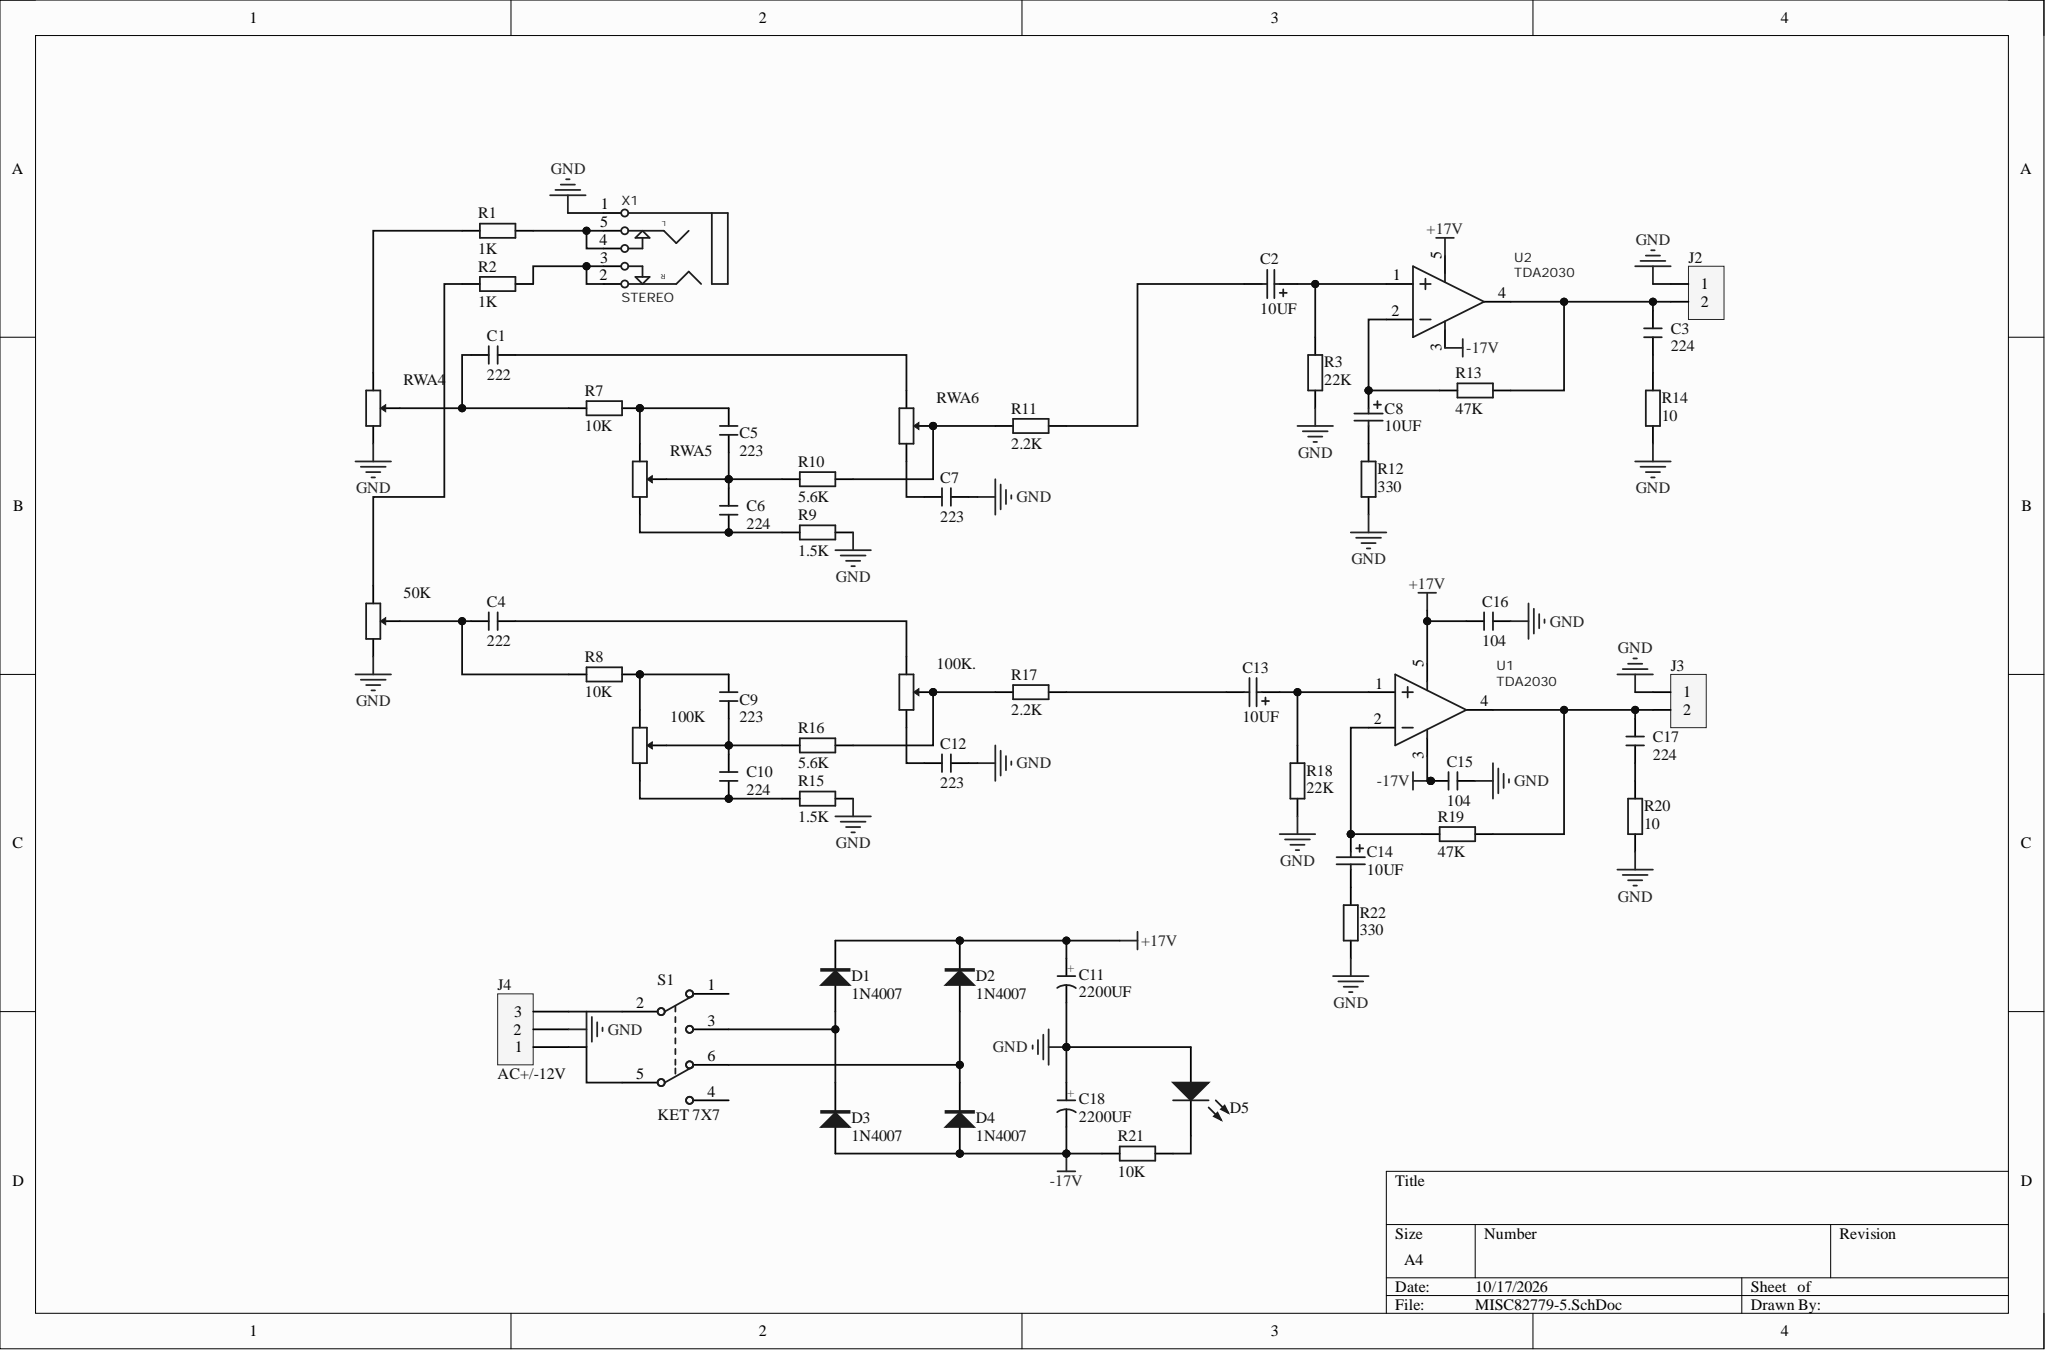Circuit board | Altium Designer | 55 parts | 38 nets
Bill of materials:
Comment,Description,Designator,Footprint,LibRef,Quantity
"10K","single-gang potentiometer","50K, 100K, 100K., RWA4, RWA5, RWA6","3296W","RP","6"
"222","ceramic disc capacitor","C1, C4","CC 2.2*5","CC","2"
"10UF","","C2, C8, C13, C14","EC100","ECAP","4"
"224","ceramic disc capacitor","C3, C6, C10, C17","CC 2.2*5","CC","4"
"223","ceramic disc capacitor","C5, C7, C9, C12","CC 2.2*5","CC","4"
"2200UF","through-hole electrolytic capacitor","C11, C18","CAP 2.5*5*11 - BK","CE","2"
"104","ceramic disc capacitor","C15, C16","CC 2.2*5","CC","2"
"1N4007","rectifier diode","D1, D2, D3, D4","DO-41","1N4007","4"
"LED","LED","D5","LED 5MM-W","LED","1"
"socket","","J2, J3","DZ","插座","2"
"AC+/-12V","","J4","VH3.96-3A","VH3","1"
"1K","color-band resistor","R1, R2","RS 1/4W","R-S","2"
"22K","color-band resistor","R3, R18","RS 1/4W","R-S","2"
"10K","color-band resistor","R7, R8, R21","RS 1/4W","R-S","3"
"1.5K","color-band resistor","R9, R15","RS 1/4W","R-S","2"
"5.6K","color-band resistor","R10, R16","RS 1/4W","R-S","2"
"2.2K","color-band resistor","R11, R17","RS 1/4W","R-S","2"
"330","color-band resistor","R12, R22","RS 1/4W","R-S","2"
"47K","color-band resistor","R13, R19","RS 1/4W","R-S","2"
"10","color-band resistor","R14, R20","RS 1/4W","R-S","2"
"KET 7X7","7*7 self-locking switch","S1","KFT DIP-7X7","KET 7X7","1"
"TDA2030","","U1, U2","TDA2030","TDA2030","2"
"STEREO","","X1","3F07","3F07","1"
Netlist (Protel format):
[
50K
3296W
10K



]
[
100K
3296W
10K



]
[
100K.
3296W
10K



]
[
C1
CC 2.2*5
222



]
[
C2
EC100
10UF



]
[
C3
CC 2.2*5
224



]
[
C4
CC 2.2*5
222



]
[
C5
CC 2.2*5
223



]
[
C6
CC 2.2*5
224



]
[
C7
CC 2.2*5
223



]
[
C8
EC100
10UF



]
[
C9
CC 2.2*5
223



]
[
C10
CC 2.2*5
224



]
[
C11
CAP 2.5*5*11 - BK
2200UF



]
[
C12
CC 2.2*5
223



]
[
C13
EC100
10UF



]
[
C14
EC100
10UF



]
[
C15
CC 2.2*5
104



]
[
C16
CC 2.2*5
104



]
[
C17
CC 2.2*5
224



]
[
C18
CAP 2.5*5*11 - BK
2200UF



]
[
D1
DO-41
1N4007



]
[
D2
DO-41
1N4007



]
[
D3
DO-41
1N4007



]
[
D4
DO-41
1N4007



]
[
D5
LED 5MM-W
LED



]
[
J2
DZ
插座



]
[
J3
DZ
插座



]
[
J4
VH3.96-3A
AC+/-12V



]
[
R1
RS 1/4W
1K



]
[
R2
RS 1/4W
1K



]
[
R3
RS 1/4W
22K



]
[
R7
RS 1/4W
10K



]
[
R8
RS 1/4W
10K



]
[
R9
RS 1/4W
1.5K



]
[
R10
RS 1/4W
5.6K



]
[
R11
RS 1/4W
2.2K



]
[
R12
RS 1/4W
330



]
[
R13
RS 1/4W
47K



]
[
R14
RS 1/4W
10



]
[
R15
RS 1/4W
1.5K



]
[
R16
RS 1/4W
5.6K



]
[
R17
RS 1/4W
2.2K



]
[
R18
RS 1/4W
22K



]
[
R19
RS 1/4W
47K



]
[
R20
RS 1/4W
10



]
[
R21
RS 1/4W
10K



]
[
R22
RS 1/4W
330



]
[
RWA4
3296W
10K



]
[
RWA5
3296W
10K



]
[
RWA6
3296W
10K



]
[
S1
KFT DIP-7X7
KET 7X7



]
[
U1
TDA2030
TDA2030



]
[
U2
TDA2030
TDA2030



]
[
X1
3F07
STEREO



]
(
Net50K_1
50K-1
R2-1
)
(
Net50K_2
50K-2
C4-1
R8-1
)
(
Net100K._1
100K.-1
C4-2
)
(
Net100K._2
100K.-2
R16-2
R17-1
)
(
Net100K._3
100K.-3
C12-2
)
(
Net100K_1
100K-1
C9-2
R8-2
)
(
Net100K_2
100K-2
C9-1
C10-2
R16-1
)
(
Net100K_3
100K-3
C10-1
R15-1
)
(
NetC1_1
C1-1
R7-1
RWA4-2
)
(
NetC1_2
C1-2
RWA6-1
)
(
NetC2_1
C2-1
R3-2
U2-1
)
(
NetC2_2
C2-2
R11-2
)
(
NetC3_1
C3-1
R14-2
)
(
NetC3_2
C3-2
J2-2
R13-1
U2-4
)
(
NetC5_1
C5-1
C6-2
R10-1
RWA5-2
)
(
NetC5_2
C5-2
R7-2
RWA5-1
)
(
NetC6_1
C6-1
R9-1
RWA5-3
)
(
NetC7_2
C7-2
RWA6-3
)
(
NetC8_1
C8-1
R13-2
U2-2
)
(
NetC8_2
C8-2
R12-2
)
(
NetC13_1
C13-1
R18-2
U1-1
)
(
NetC13_2
C13-2
R17-2
)
(
NetC14_1
C14-1
R19-2
U1-2
)
(
NetC14_2
C14-2
R22-2
)
(
NetC17_1
C17-1
R20-2
)
(
NetC17_2
C17-2
J3-2
R19-1
U1-4
)
(
NetD1_1
D1-1
D3-2
S1-3
)
(
NetD2_1
D2-1
D4-2
S1-6
)
(
NetD5_2
D5-2
R21-1
)
(
NetJ4_1
J4-1
S1-5
)
(
NetJ4_3
J4-3
S1-2
)
(
NetR1_1
R1-1
RWA4-1
)
(
NetR1_2
R1-2
X1-4
X1-5
)
(
NetR2_2
R2-2
X1-3
)
(
NetR10_2
R10-2
R11-1
RWA6-2
)
(
GND
50K-3
C7-1
C11-2
C12-1
C15-1
C16-1
C18-1
D5-1
J2-1
J3-1
J4-2
R3-1
R9-2
R12-1
R14-1
R15-2
R18-1
R20-1
R22-1
RWA4-3
X1-1
)
(
-17V
C15-2
C18-2
D3-1
D4-1
R21-2
U1-3
U2-3
)
(
+17V
C11-1
C16-2
D1-2
D2-2
U1-5
U2-5
)